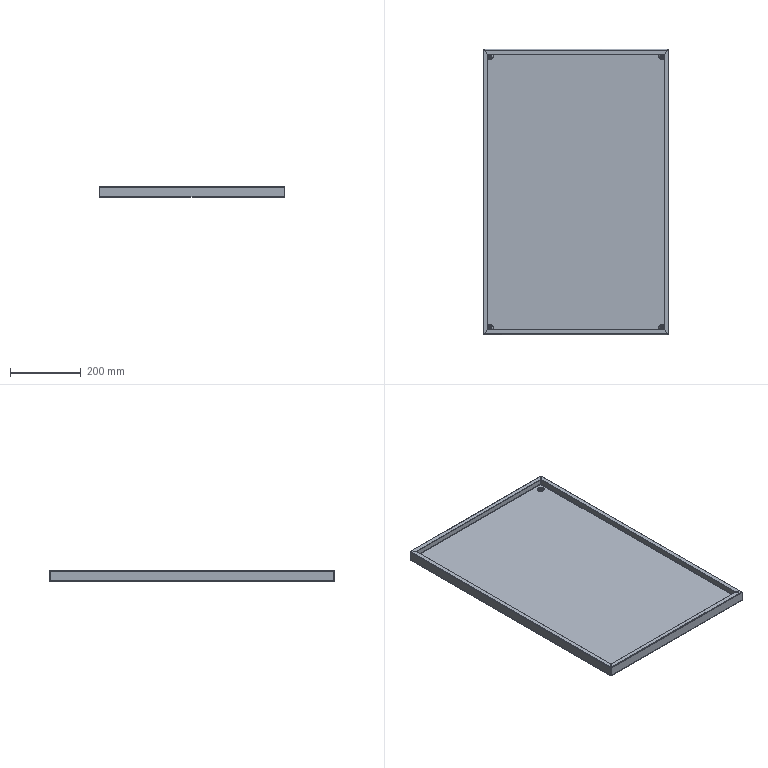Part | NX | 1 solid | 106 faces | box 524 x 804 x 30 mm | volume 786518 mm3 | plane 46 | cylinder 20 | spline 16 | torus 16 | cone 8 | commonest cylinder face diameters 1.473 x8 4.473 x8 6.5 x4